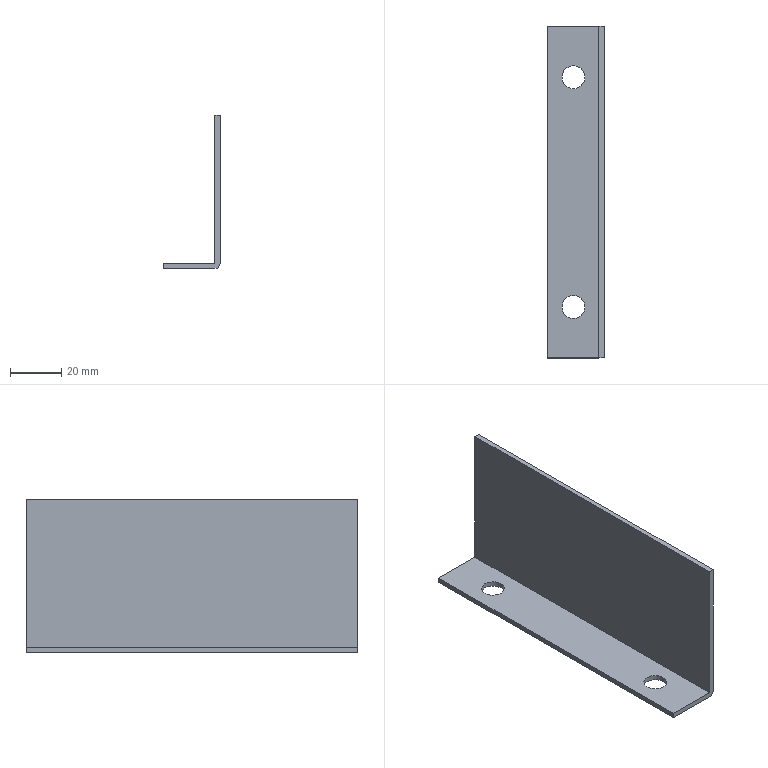Part | STEP file | lll_id4910_x_t | 1 solid | 11 faces | box 22 x 130 x 60 mm | volume 20434 mm3 | plane 8 | cylinder 3 | commonest cylinder face diameters 9 x2 4 x1
STEP:
#1=CARTESIAN_POINT('',(2260.091,-410.246,-80.));
#2=VERTEX_POINT('',#1);
#3=CARTESIAN_POINT('',(2260.091,-410.246,-78.));
#4=VERTEX_POINT('',#3);
#5=CARTESIAN_POINT('',(2260.091,-410.246,-80.));
#6=DIRECTION('',(0.,0.,1.));
#7=VECTOR('',#6,1.);
#8=LINE('',#5,#7);
#9=EDGE_CURVE('',#2,#4,#8,.T.);
#10=ORIENTED_EDGE('',*,*,#9,.T.);
#11=CARTESIAN_POINT('',(2260.091,-280.246,-78.));
#12=VERTEX_POINT('',#11);
#13=CARTESIAN_POINT('',(2260.091,-342.246,-78.));
#14=DIRECTION('',(0.,-1.,0.));
#15=VECTOR('',#14,1.);
#16=LINE('',#13,#15);
#17=EDGE_CURVE('',#12,#4,#16,.T.);
#18=ORIENTED_EDGE('',*,*,#17,.F.);
#19=CARTESIAN_POINT('',(2260.091,-280.246,-80.));
#20=VERTEX_POINT('',#19);
#21=CARTESIAN_POINT('',(2260.091,-280.246,-80.));
#22=DIRECTION('',(0.,0.,1.));
#23=VECTOR('',#22,1.);
#24=LINE('',#21,#23);
#25=EDGE_CURVE('',#20,#12,#24,.T.);
#26=ORIENTED_EDGE('',*,*,#25,.F.);
#27=CARTESIAN_POINT('',(2260.091,-342.246,-80.));
#28=DIRECTION('',(0.,-1.,0.));
#29=VECTOR('',#28,1.);
#30=LINE('',#27,#29);
#31=EDGE_CURVE('',#20,#2,#30,.T.);
#32=ORIENTED_EDGE('',*,*,#31,.T.);
#33=EDGE_LOOP('',(#10,#18,#26,#32));
#34=FACE_OUTER_BOUND('',#33,.T.);
#35=CARTESIAN_POINT('',(2260.091,-342.246,-80.));
#36=DIRECTION('',(-1.,0.,0.));
#37=DIRECTION('',(0.,-1.,0.));
#38=AXIS2_PLACEMENT_3D('',#35,#36,#37);
#39=PLANE('',#38);
#40=ADVANCED_FACE('',(#34),#39,.T.);
#41=CARTESIAN_POINT('',(2280.091,-410.246,-80.));
#42=VERTEX_POINT('',#41);
#43=CARTESIAN_POINT('',(2282.091,-410.246,-80.));
#44=DIRECTION('',(1.,0.,0.));
#45=VECTOR('',#44,1.);
#46=LINE('',#43,#45);
#47=EDGE_CURVE('',#2,#42,#46,.T.);
#48=ORIENTED_EDGE('',*,*,#47,.T.);
#49=CARTESIAN_POINT('',(2282.091,-410.246,-78.));
#50=VERTEX_POINT('',#49);
#51=CARTESIAN_POINT('',(2280.091,-410.246,-78.));
#52=DIRECTION('',(0.,-1.,0.));
#53=DIRECTION('',(0.,0.,1.));
#54=AXIS2_PLACEMENT_3D('',#51,#52,#53);
#55=CIRCLE('',#54,2.);
#56=EDGE_CURVE('',#42,#50,#55,.T.);
#57=ORIENTED_EDGE('',*,*,#56,.T.);
#58=CARTESIAN_POINT('',(2282.091,-410.246,-20.));
#59=VERTEX_POINT('',#58);
#60=CARTESIAN_POINT('',(2282.091,-410.246,-10.));
#61=DIRECTION('',(0.,0.,1.));
#62=VECTOR('',#61,1.);
#63=LINE('',#60,#62);
#64=EDGE_CURVE('',#50,#59,#63,.T.);
#65=ORIENTED_EDGE('',*,*,#64,.T.);
#66=CARTESIAN_POINT('',(2280.091,-410.246,-20.));
#67=VERTEX_POINT('',#66);
#68=CARTESIAN_POINT('',(2282.091,-410.246,-20.));
#69=DIRECTION('',(-1.,0.,0.));
#70=VECTOR('',#69,1.);
#71=LINE('',#68,#70);
#72=EDGE_CURVE('',#59,#67,#71,.T.);
#73=ORIENTED_EDGE('',*,*,#72,.T.);
#74=CARTESIAN_POINT('',(2280.091,-410.246,-78.));
#75=VERTEX_POINT('',#74);
#76=CARTESIAN_POINT('',(2280.091,-410.246,-10.));
#77=DIRECTION('',(0.,0.,1.));
#78=VECTOR('',#77,1.);
#79=LINE('',#76,#78);
#80=EDGE_CURVE('',#75,#67,#79,.T.);
#81=ORIENTED_EDGE('',*,*,#80,.F.);
#82=CARTESIAN_POINT('',(2282.091,-410.246,-78.));
#83=DIRECTION('',(1.,0.,0.));
#84=VECTOR('',#83,1.);
#85=LINE('',#82,#84);
#86=EDGE_CURVE('',#4,#75,#85,.T.);
#87=ORIENTED_EDGE('',*,*,#86,.F.);
#88=ORIENTED_EDGE('',*,*,#9,.F.);
#89=EDGE_LOOP('',(#48,#57,#65,#73,#81,#87,#88));
#90=FACE_OUTER_BOUND('',#89,.T.);
#91=CARTESIAN_POINT('',(2282.091,-410.246,-10.));
#92=DIRECTION('',(0.,1.,0.));
#93=DIRECTION('',(0.,0.,-1.));
#94=AXIS2_PLACEMENT_3D('',#91,#92,#93);
#95=PLANE('',#94);
#96=ADVANCED_FACE('',(#90),#95,.F.);
#97=CARTESIAN_POINT('',(2282.091,-280.246,-20.));
#98=VERTEX_POINT('',#97);
#99=CARTESIAN_POINT('',(2280.091,-280.246,-20.));
#100=VERTEX_POINT('',#99);
#101=CARTESIAN_POINT('',(2282.091,-280.246,-20.));
#102=DIRECTION('',(-1.,0.,0.));
#103=VECTOR('',#102,1.);
#104=LINE('',#101,#103);
#105=EDGE_CURVE('',#98,#100,#104,.T.);
#106=ORIENTED_EDGE('',*,*,#105,.T.);
#107=CARTESIAN_POINT('',(2280.091,-342.246,-20.));
#108=DIRECTION('',(0.,1.,0.));
#109=VECTOR('',#108,1.);
#110=LINE('',#107,#109);
#111=EDGE_CURVE('',#67,#100,#110,.T.);
#112=ORIENTED_EDGE('',*,*,#111,.F.);
#113=ORIENTED_EDGE('',*,*,#72,.F.);
#114=CARTESIAN_POINT('',(2282.091,-342.246,-20.));
#115=DIRECTION('',(0.,1.,0.));
#116=VECTOR('',#115,1.);
#117=LINE('',#114,#116);
#118=EDGE_CURVE('',#59,#98,#117,.T.);
#119=ORIENTED_EDGE('',*,*,#118,.T.);
#120=EDGE_LOOP('',(#106,#112,#113,#119));
#121=FACE_OUTER_BOUND('',#120,.T.);
#122=CARTESIAN_POINT('',(2282.091,-342.246,-20.));
#123=DIRECTION('',(0.,0.,-1.));
#124=DIRECTION('',(0.,-1.,0.));
#125=AXIS2_PLACEMENT_3D('',#122,#123,#124);
#126=PLANE('',#125);
#127=ADVANCED_FACE('',(#121),#126,.F.);
#128=ORIENTED_EDGE('',*,*,#111,.T.);
#129=CARTESIAN_POINT('',(2280.091,-280.246,-78.));
#130=VERTEX_POINT('',#129);
#131=CARTESIAN_POINT('',(2280.091,-280.246,-10.));
#132=DIRECTION('',(0.,0.,-1.));
#133=VECTOR('',#132,1.);
#134=LINE('',#131,#133);
#135=EDGE_CURVE('',#100,#130,#134,.T.);
#136=ORIENTED_EDGE('',*,*,#135,.T.);
#137=CARTESIAN_POINT('',(2280.091,-342.246,-78.));
#138=DIRECTION('',(0.,-1.,0.));
#139=VECTOR('',#138,1.);
#140=LINE('',#137,#139);
#141=EDGE_CURVE('',#130,#75,#140,.T.);
#142=ORIENTED_EDGE('',*,*,#141,.T.);
#143=ORIENTED_EDGE('',*,*,#80,.T.);
#144=EDGE_LOOP('',(#128,#136,#142,#143));
#145=FACE_OUTER_BOUND('',#144,.T.);
#146=CARTESIAN_POINT('',(2280.091,-342.246,-10.));
#147=DIRECTION('',(-1.,0.,0.));
#148=DIRECTION('',(0.,0.,-1.));
#149=AXIS2_PLACEMENT_3D('',#146,#147,#148);
#150=PLANE('',#149);
#151=ADVANCED_FACE('',(#145),#150,.T.);
#152=ORIENTED_EDGE('',*,*,#86,.T.);
#153=ORIENTED_EDGE('',*,*,#141,.F.);
#154=CARTESIAN_POINT('',(2282.091,-280.246,-78.));
#155=DIRECTION('',(-1.,0.,0.));
#156=VECTOR('',#155,1.);
#157=LINE('',#154,#156);
#158=EDGE_CURVE('',#130,#12,#157,.T.);
#159=ORIENTED_EDGE('',*,*,#158,.T.);
#160=ORIENTED_EDGE('',*,*,#17,.T.);
#161=EDGE_LOOP('',(#152,#153,#159,#160));
#162=FACE_BOUND('',#161,.T.);
#163=CARTESIAN_POINT('',(2270.091,-394.746,-78.));
#164=VERTEX_POINT('',#163);
#165=CARTESIAN_POINT('',(2270.091,-390.246,-78.));
#166=DIRECTION('',(0.,0.,1.));
#167=DIRECTION('',(0.,-1.,0.));
#168=AXIS2_PLACEMENT_3D('',#165,#166,#167);
#169=CIRCLE('',#168,4.5);
#170=EDGE_CURVE('',#164,#164,#169,.T.);
#171=ORIENTED_EDGE('',*,*,#170,.F.);
#172=EDGE_LOOP('',(#171));
#173=FACE_BOUND('',#172,.T.);
#174=CARTESIAN_POINT('',(2270.091,-304.746,-78.));
#175=VERTEX_POINT('',#174);
#176=CARTESIAN_POINT('',(2270.091,-300.246,-78.));
#177=DIRECTION('',(0.,0.,1.));
#178=DIRECTION('',(0.,-1.,0.));
#179=AXIS2_PLACEMENT_3D('',#176,#177,#178);
#180=CIRCLE('',#179,4.5);
#181=EDGE_CURVE('',#175,#175,#180,.T.);
#182=ORIENTED_EDGE('',*,*,#181,.F.);
#183=EDGE_LOOP('',(#182));
#184=FACE_BOUND('',#183,.T.);
#185=CARTESIAN_POINT('',(2282.091,-342.246,-78.));
#186=DIRECTION('',(0.,0.,1.));
#187=DIRECTION('',(0.,-1.,0.));
#188=AXIS2_PLACEMENT_3D('',#185,#186,#187);
#189=PLANE('',#188);
#190=ADVANCED_FACE('',(#162,#173,#184),#189,.T.);
#191=CARTESIAN_POINT('',(2282.091,-280.246,-78.));
#192=VERTEX_POINT('',#191);
#193=CARTESIAN_POINT('',(2282.091,-342.246,-78.));
#194=DIRECTION('',(0.,1.,0.));
#195=VECTOR('',#194,1.);
#196=LINE('',#193,#195);
#197=EDGE_CURVE('',#50,#192,#196,.T.);
#198=ORIENTED_EDGE('',*,*,#197,.T.);
#199=CARTESIAN_POINT('',(2282.091,-280.246,-10.));
#200=DIRECTION('',(0.,0.,-1.));
#201=VECTOR('',#200,1.);
#202=LINE('',#199,#201);
#203=EDGE_CURVE('',#98,#192,#202,.T.);
#204=ORIENTED_EDGE('',*,*,#203,.F.);
#205=ORIENTED_EDGE('',*,*,#118,.F.);
#206=ORIENTED_EDGE('',*,*,#64,.F.);
#207=EDGE_LOOP('',(#198,#204,#205,#206));
#208=FACE_OUTER_BOUND('',#207,.T.);
#209=CARTESIAN_POINT('',(2282.091,-342.246,-10.));
#210=DIRECTION('',(-1.,0.,0.));
#211=DIRECTION('',(0.,0.,-1.));
#212=AXIS2_PLACEMENT_3D('',#209,#210,#211);
#213=PLANE('',#212);
#214=ADVANCED_FACE('',(#208),#213,.F.);
#215=CARTESIAN_POINT('',(2270.091,-394.746,-80.));
#216=VERTEX_POINT('',#215);
#217=CARTESIAN_POINT('',(2270.091,-390.246,-80.));
#218=DIRECTION('',(0.,0.,1.));
#219=DIRECTION('',(0.,-1.,0.));
#220=AXIS2_PLACEMENT_3D('',#217,#218,#219);
#221=CIRCLE('',#220,4.5);
#222=EDGE_CURVE('',#216,#216,#221,.T.);
#223=ORIENTED_EDGE('',*,*,#222,.T.);
#224=EDGE_LOOP('',(#223));
#225=FACE_BOUND('',#224,.T.);
#226=ORIENTED_EDGE('',*,*,#47,.F.);
#227=ORIENTED_EDGE('',*,*,#31,.F.);
#228=CARTESIAN_POINT('',(2280.091,-280.246,-80.));
#229=VERTEX_POINT('',#228);
#230=CARTESIAN_POINT('',(2282.091,-280.246,-80.));
#231=DIRECTION('',(-1.,0.,0.));
#232=VECTOR('',#231,1.);
#233=LINE('',#230,#232);
#234=EDGE_CURVE('',#229,#20,#233,.T.);
#235=ORIENTED_EDGE('',*,*,#234,.F.);
#236=CARTESIAN_POINT('',(2280.091,-342.246,-80.));
#237=DIRECTION('',(0.,-1.,0.));
#238=VECTOR('',#237,1.);
#239=LINE('',#236,#238);
#240=EDGE_CURVE('',#229,#42,#239,.T.);
#241=ORIENTED_EDGE('',*,*,#240,.T.);
#242=EDGE_LOOP('',(#226,#227,#235,#241));
#243=FACE_BOUND('',#242,.T.);
#244=CARTESIAN_POINT('',(2270.091,-304.746,-80.));
#245=VERTEX_POINT('',#244);
#246=CARTESIAN_POINT('',(2270.091,-300.246,-80.));
#247=DIRECTION('',(0.,0.,1.));
#248=DIRECTION('',(0.,-1.,0.));
#249=AXIS2_PLACEMENT_3D('',#246,#247,#248);
#250=CIRCLE('',#249,4.5);
#251=EDGE_CURVE('',#245,#245,#250,.T.);
#252=ORIENTED_EDGE('',*,*,#251,.T.);
#253=EDGE_LOOP('',(#252));
#254=FACE_BOUND('',#253,.T.);
#255=CARTESIAN_POINT('',(2282.091,-342.246,-80.));
#256=DIRECTION('',(0.,0.,1.));
#257=DIRECTION('',(0.,-1.,0.));
#258=AXIS2_PLACEMENT_3D('',#255,#256,#257);
#259=PLANE('',#258);
#260=ADVANCED_FACE('',(#225,#243,#254),#259,.F.);
#261=ORIENTED_EDGE('',*,*,#56,.F.);
#262=ORIENTED_EDGE('',*,*,#240,.F.);
#263=CARTESIAN_POINT('',(2280.091,-280.246,-78.));
#264=DIRECTION('',(0.,1.,0.));
#265=DIRECTION('',(0.,0.,1.));
#266=AXIS2_PLACEMENT_3D('',#263,#264,#265);
#267=CIRCLE('',#266,2.);
#268=EDGE_CURVE('',#192,#229,#267,.T.);
#269=ORIENTED_EDGE('',*,*,#268,.F.);
#270=ORIENTED_EDGE('',*,*,#197,.F.);
#271=EDGE_LOOP('',(#261,#262,#269,#270));
#272=FACE_OUTER_BOUND('',#271,.T.);
#273=CARTESIAN_POINT('',(2280.091,-342.246,-78.));
#274=DIRECTION('',(0.,-1.,0.));
#275=DIRECTION('',(0.,0.,-1.));
#276=AXIS2_PLACEMENT_3D('',#273,#274,#275);
#277=CYLINDRICAL_SURFACE('',#276,2.);
#278=ADVANCED_FACE('',(#272),#277,.T.);
#279=ORIENTED_EDGE('',*,*,#170,.T.);
#280=EDGE_LOOP('',(#279));
#281=FACE_BOUND('',#280,.T.);
#282=ORIENTED_EDGE('',*,*,#222,.F.);
#283=EDGE_LOOP('',(#282));
#284=FACE_BOUND('',#283,.T.);
#285=CARTESIAN_POINT('',(2270.091,-390.246,-58.));
#286=DIRECTION('',(0.,0.,-1.));
#287=DIRECTION('',(0.,1.,0.));
#288=AXIS2_PLACEMENT_3D('',#285,#286,#287);
#289=CYLINDRICAL_SURFACE('',#288,4.5);
#290=ADVANCED_FACE('',(#281,#284),#289,.F.);
#291=ORIENTED_EDGE('',*,*,#203,.T.);
#292=ORIENTED_EDGE('',*,*,#268,.T.);
#293=ORIENTED_EDGE('',*,*,#234,.T.);
#294=ORIENTED_EDGE('',*,*,#25,.T.);
#295=ORIENTED_EDGE('',*,*,#158,.F.);
#296=ORIENTED_EDGE('',*,*,#135,.F.);
#297=ORIENTED_EDGE('',*,*,#105,.F.);
#298=EDGE_LOOP('',(#291,#292,#293,#294,#295,#296,#297));
#299=FACE_OUTER_BOUND('',#298,.T.);
#300=CARTESIAN_POINT('',(2282.091,-280.246,-80.));
#301=DIRECTION('',(0.,1.,0.));
#302=DIRECTION('',(-1.,0.,0.));
#303=AXIS2_PLACEMENT_3D('',#300,#301,#302);
#304=PLANE('',#303);
#305=ADVANCED_FACE('',(#299),#304,.T.);
#306=ORIENTED_EDGE('',*,*,#181,.T.);
#307=EDGE_LOOP('',(#306));
#308=FACE_BOUND('',#307,.T.);
#309=ORIENTED_EDGE('',*,*,#251,.F.);
#310=EDGE_LOOP('',(#309));
#311=FACE_BOUND('',#310,.T.);
#312=CARTESIAN_POINT('',(2270.091,-300.246,-58.));
#313=DIRECTION('',(0.,0.,-1.));
#314=DIRECTION('',(0.,1.,0.));
#315=AXIS2_PLACEMENT_3D('',#312,#313,#314);
#316=CYLINDRICAL_SURFACE('',#315,4.5);
#317=ADVANCED_FACE('',(#308,#311),#316,.F.);
#318=CLOSED_SHELL('',(#40,#96,#127,#151,#190,#214,#260,#278,#290,#305,#317));
#319=MANIFOLD_SOLID_BREP('',#318);
#320=(LENGTH_UNIT()NAMED_UNIT(*)SI_UNIT(.MILLI.,.METRE.));
#321=UNCERTAINTY_MEASURE_WITH_UNIT(LENGTH_MEASURE(0.00002),#320,'','');
#322=(NAMED_UNIT(*)PLANE_ANGLE_UNIT()SI_UNIT($,.RADIAN.));
#323=PLANE_ANGLE_MEASURE_WITH_UNIT(PLANE_ANGLE_MEASURE(0.01745),#322);
#324=DIMENSIONAL_EXPONENTS(0.,0.,0.,0.,0.,0.,0.);
#325=(CONVERSION_BASED_UNIT('DEGREE',#323)NAMED_UNIT(#324)PLANE_ANGLE_UNIT());
#326=(NAMED_UNIT(*)SI_UNIT($,.STERADIAN.)SOLID_ANGLE_UNIT());
#327=(GEOMETRIC_REPRESENTATION_CONTEXT(3)GLOBAL_UNCERTAINTY_ASSIGNED_CONTEXT((#321))GLOBAL_UNIT_ASSIGNED_CONTEXT((#320,#325,#326))REPRESENTATION_CONTEXT('',''));
#328=ADVANCED_BREP_SHAPE_REPRESENTATION('',(#319),#327);